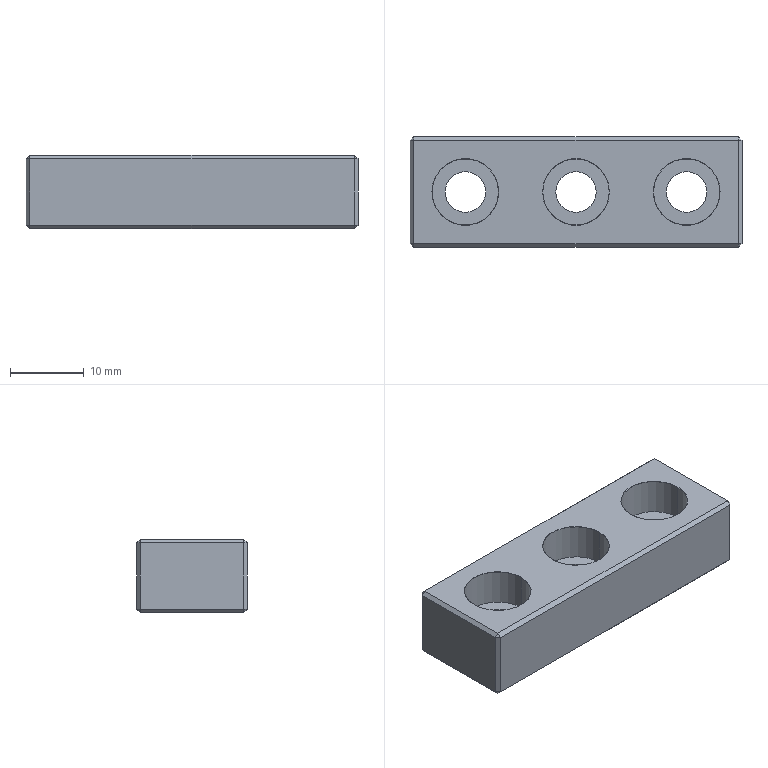Part | SolidWorks | features Chamfer 1, Extrusion 1, HoleWzd 1 | 1 solid | 47 faces | box 45 x 15 x 10 mm | volume 5405 mm3 | plane 29 | cylinder 12 | cone 6 | commonest cylinder face diameters 5.5 x6 9 x6
STEP:
#1=CARTESIAN_POINT('',(10.5,0.,9.976));
#2=VERTEX_POINT('',#1);
#3=CARTESIAN_POINT('',(19.5,0.,9.976));
#4=VERTEX_POINT('',#3);
#5=CARTESIAN_POINT('',(15.,0.,9.976));
#6=DIRECTION('',(0.,0.,1.));
#7=DIRECTION('',(1.,0.,0.));
#8=AXIS2_PLACEMENT_3D('',#5,#6,#7);
#9=CIRCLE('',#8,4.5);
#10=EDGE_CURVE('',#2,#4,#9,.T.);
#11=ORIENTED_EDGE('',*,*,#10,.F.);
#12=CARTESIAN_POINT('',(10.475,0.,10.));
#13=VERTEX_POINT('',#12);
#14=CARTESIAN_POINT('',(10.475,0.,10.));
#15=DIRECTION('',(-0.7193,0.,0.6947));
#16=VECTOR('',#15,1000.);
#17=LINE('',#14,#16);
#18=EDGE_CURVE('',#2,#13,#17,.T.);
#19=ORIENTED_EDGE('',*,*,#18,.T.);
#20=CARTESIAN_POINT('',(19.525,0.,10.));
#21=VERTEX_POINT('',#20);
#22=CARTESIAN_POINT('',(15.,0.,10.));
#23=DIRECTION('',(0.,0.,1.));
#24=DIRECTION('',(1.,0.,0.));
#25=AXIS2_PLACEMENT_3D('',#22,#23,#24);
#26=CIRCLE('',#25,4.525);
#27=EDGE_CURVE('',#13,#21,#26,.T.);
#28=ORIENTED_EDGE('',*,*,#27,.T.);
#29=CARTESIAN_POINT('',(19.525,0.,10.));
#30=DIRECTION('',(0.7193,0.,0.6947));
#31=VECTOR('',#30,1000.);
#32=LINE('',#29,#31);
#33=EDGE_CURVE('',#4,#21,#32,.T.);
#34=ORIENTED_EDGE('',*,*,#33,.F.);
#35=EDGE_LOOP('',(#11,#19,#28,#34));
#36=FACE_OUTER_BOUND('',#35,.T.);
#37=CARTESIAN_POINT('',(15.,0.,10.));
#38=DIRECTION('',(0.,0.,1.));
#39=DIRECTION('',(1.,0.,0.));
#40=AXIS2_PLACEMENT_3D('',#37,#38,#39);
#41=CONICAL_SURFACE('',#40,4.525,0.8029);
#42=ADVANCED_FACE('',(#36),#41,.F.);
#43=CARTESIAN_POINT('',(10.5,0.,5.));
#44=VERTEX_POINT('',#43);
#45=CARTESIAN_POINT('',(19.5,0.,5.));
#46=VERTEX_POINT('',#45);
#47=CARTESIAN_POINT('',(15.,0.,5.));
#48=DIRECTION('',(0.,0.,1.));
#49=DIRECTION('',(1.,0.,0.));
#50=AXIS2_PLACEMENT_3D('',#47,#48,#49);
#51=CIRCLE('',#50,4.5);
#52=EDGE_CURVE('',#44,#46,#51,.T.);
#53=ORIENTED_EDGE('',*,*,#52,.F.);
#54=CARTESIAN_POINT('',(10.5,0.,10.));
#55=DIRECTION('',(0.,0.,1.));
#56=VECTOR('',#55,1000.);
#57=LINE('',#54,#56);
#58=EDGE_CURVE('',#44,#2,#57,.T.);
#59=ORIENTED_EDGE('',*,*,#58,.T.);
#60=ORIENTED_EDGE('',*,*,#10,.T.);
#61=CARTESIAN_POINT('',(19.5,0.,10.));
#62=DIRECTION('',(0.,0.,1.));
#63=VECTOR('',#62,1000.);
#64=LINE('',#61,#63);
#65=EDGE_CURVE('',#46,#4,#64,.T.);
#66=ORIENTED_EDGE('',*,*,#65,.F.);
#67=EDGE_LOOP('',(#53,#59,#60,#66));
#68=FACE_OUTER_BOUND('',#67,.T.);
#69=CARTESIAN_POINT('',(15.,0.,10.));
#70=DIRECTION('',(0.,0.,1.));
#71=DIRECTION('',(1.,0.,0.));
#72=AXIS2_PLACEMENT_3D('',#69,#70,#71);
#73=CYLINDRICAL_SURFACE('',#72,4.5);
#74=ADVANCED_FACE('',(#68),#73,.F.);
#75=CARTESIAN_POINT('',(12.25,0.,0.));
#76=VERTEX_POINT('',#75);
#77=CARTESIAN_POINT('',(17.75,0.,0.));
#78=VERTEX_POINT('',#77);
#79=CARTESIAN_POINT('',(15.,0.,0.));
#80=DIRECTION('',(0.,0.,1.));
#81=DIRECTION('',(1.,0.,0.));
#82=AXIS2_PLACEMENT_3D('',#79,#80,#81);
#83=CIRCLE('',#82,2.75);
#84=EDGE_CURVE('',#76,#78,#83,.T.);
#85=ORIENTED_EDGE('',*,*,#84,.F.);
#86=CARTESIAN_POINT('',(12.25,0.,5.));
#87=VERTEX_POINT('',#86);
#88=CARTESIAN_POINT('',(12.25,0.,10.));
#89=DIRECTION('',(0.,0.,1.));
#90=VECTOR('',#89,1000.);
#91=LINE('',#88,#90);
#92=EDGE_CURVE('',#76,#87,#91,.T.);
#93=ORIENTED_EDGE('',*,*,#92,.T.);
#94=CARTESIAN_POINT('',(17.75,0.,5.));
#95=VERTEX_POINT('',#94);
#96=CARTESIAN_POINT('',(15.,0.,5.));
#97=DIRECTION('',(0.,0.,1.));
#98=DIRECTION('',(1.,0.,0.));
#99=AXIS2_PLACEMENT_3D('',#96,#97,#98);
#100=CIRCLE('',#99,2.75);
#101=EDGE_CURVE('',#87,#95,#100,.T.);
#102=ORIENTED_EDGE('',*,*,#101,.T.);
#103=CARTESIAN_POINT('',(17.75,0.,10.));
#104=DIRECTION('',(0.,0.,1.));
#105=VECTOR('',#104,1000.);
#106=LINE('',#103,#105);
#107=EDGE_CURVE('',#78,#95,#106,.T.);
#108=ORIENTED_EDGE('',*,*,#107,.F.);
#109=EDGE_LOOP('',(#85,#93,#102,#108));
#110=FACE_OUTER_BOUND('',#109,.T.);
#111=CARTESIAN_POINT('',(15.,0.,10.));
#112=DIRECTION('',(0.,0.,1.));
#113=DIRECTION('',(1.,0.,0.));
#114=AXIS2_PLACEMENT_3D('',#111,#112,#113);
#115=CYLINDRICAL_SURFACE('',#114,2.75);
#116=ADVANCED_FACE('',(#110),#115,.F.);
#117=CARTESIAN_POINT('',(-19.5,0.,9.976));
#118=VERTEX_POINT('',#117);
#119=CARTESIAN_POINT('',(-10.5,0.,9.976));
#120=VERTEX_POINT('',#119);
#121=CARTESIAN_POINT('',(-15.,0.,9.976));
#122=DIRECTION('',(0.,0.,1.));
#123=DIRECTION('',(1.,0.,0.));
#124=AXIS2_PLACEMENT_3D('',#121,#122,#123);
#125=CIRCLE('',#124,4.5);
#126=EDGE_CURVE('',#118,#120,#125,.T.);
#127=ORIENTED_EDGE('',*,*,#126,.F.);
#128=CARTESIAN_POINT('',(-19.525,0.,10.));
#129=VERTEX_POINT('',#128);
#130=CARTESIAN_POINT('',(-19.525,0.,10.));
#131=DIRECTION('',(-0.7193,0.,0.6947));
#132=VECTOR('',#131,1000.);
#133=LINE('',#130,#132);
#134=EDGE_CURVE('',#118,#129,#133,.T.);
#135=ORIENTED_EDGE('',*,*,#134,.T.);
#136=CARTESIAN_POINT('',(-10.475,0.,10.));
#137=VERTEX_POINT('',#136);
#138=CARTESIAN_POINT('',(-15.,0.,10.));
#139=DIRECTION('',(0.,0.,1.));
#140=DIRECTION('',(1.,0.,0.));
#141=AXIS2_PLACEMENT_3D('',#138,#139,#140);
#142=CIRCLE('',#141,4.525);
#143=EDGE_CURVE('',#129,#137,#142,.T.);
#144=ORIENTED_EDGE('',*,*,#143,.T.);
#145=CARTESIAN_POINT('',(-10.475,0.,10.));
#146=DIRECTION('',(0.7193,0.,0.6947));
#147=VECTOR('',#146,1000.);
#148=LINE('',#145,#147);
#149=EDGE_CURVE('',#120,#137,#148,.T.);
#150=ORIENTED_EDGE('',*,*,#149,.F.);
#151=EDGE_LOOP('',(#127,#135,#144,#150));
#152=FACE_OUTER_BOUND('',#151,.T.);
#153=CARTESIAN_POINT('',(-15.,0.,10.));
#154=DIRECTION('',(0.,0.,1.));
#155=DIRECTION('',(1.,0.,0.));
#156=AXIS2_PLACEMENT_3D('',#153,#154,#155);
#157=CONICAL_SURFACE('',#156,4.525,0.8029);
#158=ADVANCED_FACE('',(#152),#157,.F.);
#159=CARTESIAN_POINT('',(-19.5,0.,5.));
#160=VERTEX_POINT('',#159);
#161=CARTESIAN_POINT('',(-10.5,0.,5.));
#162=VERTEX_POINT('',#161);
#163=CARTESIAN_POINT('',(-15.,0.,5.));
#164=DIRECTION('',(0.,0.,1.));
#165=DIRECTION('',(1.,0.,0.));
#166=AXIS2_PLACEMENT_3D('',#163,#164,#165);
#167=CIRCLE('',#166,4.5);
#168=EDGE_CURVE('',#160,#162,#167,.T.);
#169=ORIENTED_EDGE('',*,*,#168,.F.);
#170=CARTESIAN_POINT('',(-19.5,0.,10.));
#171=DIRECTION('',(0.,0.,1.));
#172=VECTOR('',#171,1000.);
#173=LINE('',#170,#172);
#174=EDGE_CURVE('',#160,#118,#173,.T.);
#175=ORIENTED_EDGE('',*,*,#174,.T.);
#176=ORIENTED_EDGE('',*,*,#126,.T.);
#177=CARTESIAN_POINT('',(-10.5,0.,10.));
#178=DIRECTION('',(0.,0.,1.));
#179=VECTOR('',#178,1000.);
#180=LINE('',#177,#179);
#181=EDGE_CURVE('',#162,#120,#180,.T.);
#182=ORIENTED_EDGE('',*,*,#181,.F.);
#183=EDGE_LOOP('',(#169,#175,#176,#182));
#184=FACE_OUTER_BOUND('',#183,.T.);
#185=CARTESIAN_POINT('',(-15.,0.,10.));
#186=DIRECTION('',(0.,0.,1.));
#187=DIRECTION('',(1.,0.,0.));
#188=AXIS2_PLACEMENT_3D('',#185,#186,#187);
#189=CYLINDRICAL_SURFACE('',#188,4.5);
#190=ADVANCED_FACE('',(#184),#189,.F.);
#191=CARTESIAN_POINT('',(-17.75,0.,0.));
#192=VERTEX_POINT('',#191);
#193=CARTESIAN_POINT('',(-12.25,0.,0.));
#194=VERTEX_POINT('',#193);
#195=CARTESIAN_POINT('',(-15.,0.,0.));
#196=DIRECTION('',(0.,0.,1.));
#197=DIRECTION('',(1.,0.,0.));
#198=AXIS2_PLACEMENT_3D('',#195,#196,#197);
#199=CIRCLE('',#198,2.75);
#200=EDGE_CURVE('',#192,#194,#199,.T.);
#201=ORIENTED_EDGE('',*,*,#200,.F.);
#202=CARTESIAN_POINT('',(-17.75,0.,5.));
#203=VERTEX_POINT('',#202);
#204=CARTESIAN_POINT('',(-17.75,0.,10.));
#205=DIRECTION('',(0.,0.,1.));
#206=VECTOR('',#205,1000.);
#207=LINE('',#204,#206);
#208=EDGE_CURVE('',#192,#203,#207,.T.);
#209=ORIENTED_EDGE('',*,*,#208,.T.);
#210=CARTESIAN_POINT('',(-12.25,0.,5.));
#211=VERTEX_POINT('',#210);
#212=CARTESIAN_POINT('',(-15.,0.,5.));
#213=DIRECTION('',(0.,0.,1.));
#214=DIRECTION('',(1.,0.,0.));
#215=AXIS2_PLACEMENT_3D('',#212,#213,#214);
#216=CIRCLE('',#215,2.75);
#217=EDGE_CURVE('',#203,#211,#216,.T.);
#218=ORIENTED_EDGE('',*,*,#217,.T.);
#219=CARTESIAN_POINT('',(-12.25,0.,10.));
#220=DIRECTION('',(0.,0.,1.));
#221=VECTOR('',#220,1000.);
#222=LINE('',#219,#221);
#223=EDGE_CURVE('',#194,#211,#222,.T.);
#224=ORIENTED_EDGE('',*,*,#223,.F.);
#225=EDGE_LOOP('',(#201,#209,#218,#224));
#226=FACE_OUTER_BOUND('',#225,.T.);
#227=CARTESIAN_POINT('',(-15.,0.,10.));
#228=DIRECTION('',(0.,0.,1.));
#229=DIRECTION('',(1.,0.,0.));
#230=AXIS2_PLACEMENT_3D('',#227,#228,#229);
#231=CYLINDRICAL_SURFACE('',#230,2.75);
#232=ADVANCED_FACE('',(#226),#231,.F.);
#233=CARTESIAN_POINT('',(-4.5,0.,9.976));
#234=VERTEX_POINT('',#233);
#235=CARTESIAN_POINT('',(4.5,0.,9.976));
#236=VERTEX_POINT('',#235);
#237=CARTESIAN_POINT('',(0.,0.,9.976));
#238=DIRECTION('',(0.,0.,1.));
#239=DIRECTION('',(1.,0.,0.));
#240=AXIS2_PLACEMENT_3D('',#237,#238,#239);
#241=CIRCLE('',#240,4.5);
#242=EDGE_CURVE('',#234,#236,#241,.T.);
#243=ORIENTED_EDGE('',*,*,#242,.F.);
#244=CARTESIAN_POINT('',(-4.525,0.,10.));
#245=VERTEX_POINT('',#244);
#246=CARTESIAN_POINT('',(-4.525,0.,10.));
#247=DIRECTION('',(-0.7193,0.,0.6947));
#248=VECTOR('',#247,1000.);
#249=LINE('',#246,#248);
#250=EDGE_CURVE('',#234,#245,#249,.T.);
#251=ORIENTED_EDGE('',*,*,#250,.T.);
#252=CARTESIAN_POINT('',(4.525,0.,10.));
#253=VERTEX_POINT('',#252);
#254=CARTESIAN_POINT('',(0.,0.,10.));
#255=DIRECTION('',(0.,0.,1.));
#256=DIRECTION('',(1.,0.,0.));
#257=AXIS2_PLACEMENT_3D('',#254,#255,#256);
#258=CIRCLE('',#257,4.525);
#259=EDGE_CURVE('',#245,#253,#258,.T.);
#260=ORIENTED_EDGE('',*,*,#259,.T.);
#261=CARTESIAN_POINT('',(4.525,0.,10.));
#262=DIRECTION('',(0.7193,0.,0.6947));
#263=VECTOR('',#262,1000.);
#264=LINE('',#261,#263);
#265=EDGE_CURVE('',#236,#253,#264,.T.);
#266=ORIENTED_EDGE('',*,*,#265,.F.);
#267=EDGE_LOOP('',(#243,#251,#260,#266));
#268=FACE_OUTER_BOUND('',#267,.T.);
#269=CARTESIAN_POINT('',(0.,0.,10.));
#270=DIRECTION('',(0.,0.,1.));
#271=DIRECTION('',(1.,0.,0.));
#272=AXIS2_PLACEMENT_3D('',#269,#270,#271);
#273=CONICAL_SURFACE('',#272,4.525,0.8029);
#274=ADVANCED_FACE('',(#268),#273,.F.);
#275=CARTESIAN_POINT('',(-4.5,0.,5.));
#276=VERTEX_POINT('',#275);
#277=CARTESIAN_POINT('',(4.5,0.,5.));
#278=VERTEX_POINT('',#277);
#279=CARTESIAN_POINT('',(0.,0.,5.));
#280=DIRECTION('',(0.,0.,1.));
#281=DIRECTION('',(1.,0.,0.));
#282=AXIS2_PLACEMENT_3D('',#279,#280,#281);
#283=CIRCLE('',#282,4.5);
#284=EDGE_CURVE('',#276,#278,#283,.T.);
#285=ORIENTED_EDGE('',*,*,#284,.F.);
#286=CARTESIAN_POINT('',(-4.5,0.,10.));
#287=DIRECTION('',(0.,0.,1.));
#288=VECTOR('',#287,1000.);
#289=LINE('',#286,#288);
#290=EDGE_CURVE('',#276,#234,#289,.T.);
#291=ORIENTED_EDGE('',*,*,#290,.T.);
#292=ORIENTED_EDGE('',*,*,#242,.T.);
#293=CARTESIAN_POINT('',(4.5,0.,10.));
#294=DIRECTION('',(0.,0.,1.));
#295=VECTOR('',#294,1000.);
#296=LINE('',#293,#295);
#297=EDGE_CURVE('',#278,#236,#296,.T.);
#298=ORIENTED_EDGE('',*,*,#297,.F.);
#299=EDGE_LOOP('',(#285,#291,#292,#298));
#300=FACE_OUTER_BOUND('',#299,.T.);
#301=CARTESIAN_POINT('',(0.,0.,10.));
#302=DIRECTION('',(0.,0.,1.));
#303=DIRECTION('',(1.,0.,0.));
#304=AXIS2_PLACEMENT_3D('',#301,#302,#303);
#305=CYLINDRICAL_SURFACE('',#304,4.5);
#306=ADVANCED_FACE('',(#300),#305,.F.);
#307=CARTESIAN_POINT('',(-2.75,0.,0.));
#308=VERTEX_POINT('',#307);
#309=CARTESIAN_POINT('',(2.75,0.,0.));
#310=VERTEX_POINT('',#309);
#311=CARTESIAN_POINT('',(0.,0.,0.));
#312=DIRECTION('',(0.,0.,1.));
#313=DIRECTION('',(1.,0.,0.));
#314=AXIS2_PLACEMENT_3D('',#311,#312,#313);
#315=CIRCLE('',#314,2.75);
#316=EDGE_CURVE('',#308,#310,#315,.T.);
#317=ORIENTED_EDGE('',*,*,#316,.F.);
#318=CARTESIAN_POINT('',(-2.75,0.,5.));
#319=VERTEX_POINT('',#318);
#320=CARTESIAN_POINT('',(-2.75,0.,10.));
#321=DIRECTION('',(0.,0.,1.));
#322=VECTOR('',#321,1000.);
#323=LINE('',#320,#322);
#324=EDGE_CURVE('',#308,#319,#323,.T.);
#325=ORIENTED_EDGE('',*,*,#324,.T.);
#326=CARTESIAN_POINT('',(2.75,0.,5.));
#327=VERTEX_POINT('',#326);
#328=CARTESIAN_POINT('',(0.,0.,5.));
#329=DIRECTION('',(0.,0.,1.));
#330=DIRECTION('',(1.,0.,0.));
#331=AXIS2_PLACEMENT_3D('',#328,#329,#330);
#332=CIRCLE('',#331,2.75);
#333=EDGE_CURVE('',#319,#327,#332,.T.);
#334=ORIENTED_EDGE('',*,*,#333,.T.);
#335=CARTESIAN_POINT('',(2.75,0.,10.));
#336=DIRECTION('',(0.,0.,1.));
#337=VECTOR('',#336,1000.);
#338=LINE('',#335,#337);
#339=EDGE_CURVE('',#310,#327,#338,.T.);
#340=ORIENTED_EDGE('',*,*,#339,.F.);
#341=EDGE_LOOP('',(#317,#325,#334,#340));
#342=FACE_OUTER_BOUND('',#341,.T.);
#343=CARTESIAN_POINT('',(0.,0.,10.));
#344=DIRECTION('',(0.,0.,1.));
#345=DIRECTION('',(1.,0.,0.));
#346=AXIS2_PLACEMENT_3D('',#343,#344,#345);
#347=CYLINDRICAL_SURFACE('',#346,2.75);
#348=ADVANCED_FACE('',(#342),#347,.F.);
#349=CARTESIAN_POINT('',(22.5,7.,0.5));
#350=VERTEX_POINT('',#349);
#351=CARTESIAN_POINT('',(22.5,7.,9.5));
#352=VERTEX_POINT('',#351);
#353=CARTESIAN_POINT('',(22.5,7.,10.));
#354=DIRECTION('',(0.,0.,1.));
#355=VECTOR('',#354,1000.);
#356=LINE('',#353,#355);
#357=EDGE_CURVE('',#350,#352,#356,.T.);
#358=ORIENTED_EDGE('',*,*,#357,.T.);
#359=CARTESIAN_POINT('',(22.5,-7.,9.5));
#360=VERTEX_POINT('',#359);
#361=CARTESIAN_POINT('',(22.5,-7.5,9.5));
#362=DIRECTION('',(0.,-1.,0.));
#363=VECTOR('',#362,1000.);
#364=LINE('',#361,#363);
#365=EDGE_CURVE('',#352,#360,#364,.T.);
#366=ORIENTED_EDGE('',*,*,#365,.T.);
#367=CARTESIAN_POINT('',(22.5,-7.,0.5));
#368=VERTEX_POINT('',#367);
#369=CARTESIAN_POINT('',(22.5,-7.,10.));
#370=DIRECTION('',(0.,0.,-1.));
#371=VECTOR('',#370,1000.);
#372=LINE('',#369,#371);
#373=EDGE_CURVE('',#360,#368,#372,.T.);
#374=ORIENTED_EDGE('',*,*,#373,.T.);
#375=CARTESIAN_POINT('',(22.5,7.5,0.5));
#376=DIRECTION('',(0.,1.,0.));
#377=VECTOR('',#376,1000.);
#378=LINE('',#375,#377);
#379=EDGE_CURVE('',#368,#350,#378,.T.);
#380=ORIENTED_EDGE('',*,*,#379,.T.);
#381=EDGE_LOOP('',(#358,#366,#374,#380));
#382=FACE_OUTER_BOUND('',#381,.T.);
#383=CARTESIAN_POINT('',(22.5,7.5,10.));
#384=DIRECTION('',(-1.,0.,0.));
#385=DIRECTION('',(0.,-1.,0.));
#386=AXIS2_PLACEMENT_3D('',#383,#384,#385);
#387=PLANE('',#386);
#388=ADVANCED_FACE('',(#382),#387,.F.);
#389=CARTESIAN_POINT('',(-22.,7.5,9.5));
#390=VERTEX_POINT('',#389);
#391=CARTESIAN_POINT('',(22.,7.5,9.5));
#392=VERTEX_POINT('',#391);
#393=CARTESIAN_POINT('',(22.5,7.5,9.5));
#394=DIRECTION('',(1.,0.,0.));
#395=VECTOR('',#394,1000.);
#396=LINE('',#393,#395);
#397=EDGE_CURVE('',#390,#392,#396,.T.);
#398=ORIENTED_EDGE('',*,*,#397,.T.);
#399=CARTESIAN_POINT('',(22.,7.5,0.5));
#400=VERTEX_POINT('',#399);
#401=CARTESIAN_POINT('',(22.,7.5,10.));
#402=DIRECTION('',(0.,0.,-1.));
#403=VECTOR('',#402,1000.);
#404=LINE('',#401,#403);
#405=EDGE_CURVE('',#392,#400,#404,.T.);
#406=ORIENTED_EDGE('',*,*,#405,.T.);
#407=CARTESIAN_POINT('',(-22.,7.5,0.5));
#408=VERTEX_POINT('',#407);
#409=CARTESIAN_POINT('',(-22.5,7.5,0.5));
#410=DIRECTION('',(-1.,0.,0.));
#411=VECTOR('',#410,1000.);
#412=LINE('',#409,#411);
#413=EDGE_CURVE('',#400,#408,#412,.T.);
#414=ORIENTED_EDGE('',*,*,#413,.T.);
#415=CARTESIAN_POINT('',(-22.,7.5,10.));
#416=DIRECTION('',(0.,0.,1.));
#417=VECTOR('',#416,1000.);
#418=LINE('',#415,#417);
#419=EDGE_CURVE('',#408,#390,#418,.T.);
#420=ORIENTED_EDGE('',*,*,#419,.T.);
#421=EDGE_LOOP('',(#398,#406,#414,#420));
#422=FACE_OUTER_BOUND('',#421,.T.);
#423=CARTESIAN_POINT('',(-22.5,7.5,10.));
#424=DIRECTION('',(0.,-1.,0.));
#425=DIRECTION('',(0.,0.,-1.));
#426=AXIS2_PLACEMENT_3D('',#423,#424,#425);
#427=PLANE('',#426);
#428=ADVANCED_FACE('',(#422),#427,.F.);
#429=CARTESIAN_POINT('',(-22.5,7.,0.5));
#430=VERTEX_POINT('',#429);
#431=CARTESIAN_POINT('',(-22.5,-7.,0.5));
#432=VERTEX_POINT('',#431);
#433=CARTESIAN_POINT('',(-22.5,7.5,0.5));
#434=DIRECTION('',(0.,-1.,0.));
#435=VECTOR('',#434,1000.);
#436=LINE('',#433,#435);
#437=EDGE_CURVE('',#430,#432,#436,.T.);
#438=ORIENTED_EDGE('',*,*,#437,.T.);
#439=CARTESIAN_POINT('',(-22.5,-7.,9.5));
#440=VERTEX_POINT('',#439);
#441=CARTESIAN_POINT('',(-22.5,-7.,10.));
#442=DIRECTION('',(0.,0.,1.));
#443=VECTOR('',#442,1000.);
#444=LINE('',#441,#443);
#445=EDGE_CURVE('',#432,#440,#444,.T.);
#446=ORIENTED_EDGE('',*,*,#445,.T.);
#447=CARTESIAN_POINT('',(-22.5,7.,9.5));
#448=VERTEX_POINT('',#447);
#449=CARTESIAN_POINT('',(-22.5,7.5,9.5));
#450=DIRECTION('',(0.,1.,0.));
#451=VECTOR('',#450,1000.);
#452=LINE('',#449,#451);
#453=EDGE_CURVE('',#440,#448,#452,.T.);
#454=ORIENTED_EDGE('',*,*,#453,.T.);
#455=CARTESIAN_POINT('',(-22.5,7.,10.));
#456=DIRECTION('',(0.,0.,-1.));
#457=VECTOR('',#456,1000.);
#458=LINE('',#455,#457);
#459=EDGE_CURVE('',#448,#430,#458,.T.);
#460=ORIENTED_EDGE('',*,*,#459,.T.);
#461=EDGE_LOOP('',(#438,#446,#454,#460));
#462=FACE_OUTER_BOUND('',#461,.T.);
#463=CARTESIAN_POINT('',(-22.5,7.5,10.));
#464=DIRECTION('',(1.,0.,0.));
#465=DIRECTION('',(0.,0.,-1.));
#466=AXIS2_PLACEMENT_3D('',#463,#464,#465);
#467=PLANE('',#466);
#468=ADVANCED_FACE('',(#462),#467,.F.);
#469=CARTESIAN_POINT('',(22.,-7.5,9.5));
#470=VERTEX_POINT('',#469);
#471=CARTESIAN_POINT('',(-22.,-7.5,9.5));
#472=VERTEX_POINT('',#471);
#473=CARTESIAN_POINT('',(-22.5,-7.5,9.5));
#474=DIRECTION('',(-1.,0.,0.));
#475=VECTOR('',#474,1000.);
#476=LINE('',#473,#475);
#477=EDGE_CURVE('',#470,#472,#476,.T.);
#478=ORIENTED_EDGE('',*,*,#477,.T.);
#479=CARTESIAN_POINT('',(-22.,-7.5,0.5));
#480=VERTEX_POINT('',#479);
#481=CARTESIAN_POINT('',(-22.,-7.5,10.));
#482=DIRECTION('',(0.,0.,-1.));
#483=VECTOR('',#482,1000.);
#484=LINE('',#481,#483);
#485=EDGE_CURVE('',#472,#480,#484,.T.);
#486=ORIENTED_EDGE('',*,*,#485,.T.);
#487=CARTESIAN_POINT('',(22.,-7.5,0.5));
#488=VERTEX_POINT('',#487);
#489=CARTESIAN_POINT('',(-22.5,-7.5,0.5));
#490=DIRECTION('',(1.,0.,0.));
#491=VECTOR('',#490,1000.);
#492=LINE('',#489,#491);
#493=EDGE_CURVE('',#480,#488,#492,.T.);
#494=ORIENTED_EDGE('',*,*,#493,.T.);
#495=CARTESIAN_POINT('',(22.,-7.5,10.));
#496=DIRECTION('',(0.,0.,1.));
#497=VECTOR('',#496,1000.);
#498=LINE('',#495,#497);
#499=EDGE_CURVE('',#488,#470,#498,.T.);
#500=ORIENTED_EDGE('',*,*,#499,.T.);
#501=EDGE_LOOP('',(#478,#486,#494,#500));
#502=FACE_OUTER_BOUND('',#501,.T.);
#503=CARTESIAN_POINT('',(-22.5,-7.5,10.));
#504=DIRECTION('',(0.,1.,0.));
#505=DIRECTION('',(0.,0.,1.));
#506=AXIS2_PLACEMENT_3D('',#503,#504,#505);
#507=PLANE('',#506);
#508=ADVANCED_FACE('',(#502),#507,.F.);
#509=CARTESIAN_POINT('',(-22.,7.,10.));
#510=VERTEX_POINT('',#509);
#511=CARTESIAN_POINT('',(-22.,-7.,10.));
#512=VERTEX_POINT('',#511);
#513=CARTESIAN_POINT('',(-22.,-7.5,10.));
#514=DIRECTION('',(0.,-1.,0.));
#515=VECTOR('',#514,1000.);
#516=LINE('',#513,#515);
#517=EDGE_CURVE('',#510,#512,#516,.T.);
#518=ORIENTED_EDGE('',*,*,#517,.T.);
#519=CARTESIAN_POINT('',(22.,-7.,10.));
#520=VERTEX_POINT('',#519);
#521=CARTESIAN_POINT('',(22.5,-7.,10.));
#522=DIRECTION('',(1.,0.,0.));
#523=VECTOR('',#522,1000.);
#524=LINE('',#521,#523);
#525=EDGE_CURVE('',#512,#520,#524,.T.);
#526=ORIENTED_EDGE('',*,*,#525,.T.);
#527=CARTESIAN_POINT('',(22.,7.,10.));
#528=VERTEX_POINT('',#527);
#529=CARTESIAN_POINT('',(22.,7.5,10.));
#530=DIRECTION('',(0.,1.,0.));
#531=VECTOR('',#530,1000.);
#532=LINE('',#529,#531);
#533=EDGE_CURVE('',#520,#528,#532,.T.);
#534=ORIENTED_EDGE('',*,*,#533,.T.);
#535=CARTESIAN_POINT('',(-22.5,7.,10.));
#536=DIRECTION('',(-1.,0.,0.));
#537=VECTOR('',#536,1000.);
#538=LINE('',#535,#537);
#539=EDGE_CURVE('',#528,#510,#538,.T.);
#540=ORIENTED_EDGE('',*,*,#539,.T.);
#541=EDGE_LOOP('',(#518,#526,#534,#540));
#542=FACE_OUTER_BOUND('',#541,.T.);
#543=CARTESIAN_POINT('',(15.,0.,10.));
#544=DIRECTION('',(0.,0.,1.));
#545=DIRECTION('',(1.,0.,0.));
#546=AXIS2_PLACEMENT_3D('',#543,#544,#545);
#547=CIRCLE('',#546,4.525);
#548=EDGE_CURVE('',#21,#13,#547,.T.);
#549=ORIENTED_EDGE('',*,*,#548,.F.);
#550=ORIENTED_EDGE('',*,*,#27,.F.);
#551=EDGE_LOOP('',(#549,#550));
#552=FACE_BOUND('',#551,.T.);
#553=CARTESIAN_POINT('',(-15.,0.,10.));
#554=DIRECTION('',(0.,0.,1.));
#555=DIRECTION('',(1.,0.,0.));
#556=AXIS2_PLACEMENT_3D('',#553,#554,#555);
#557=CIRCLE('',#556,4.525);
#558=EDGE_CURVE('',#137,#129,#557,.T.);
#559=ORIENTED_EDGE('',*,*,#558,.F.);
#560=ORIENTED_EDGE('',*,*,#143,.F.);
#561=EDGE_LOOP('',(#559,#560));
#562=FACE_BOUND('',#561,.T.);
#563=CARTESIAN_POINT('',(0.,0.,10.));
#564=DIRECTION('',(0.,0.,1.));
#565=DIRECTION('',(1.,0.,0.));
#566=AXIS2_PLACEMENT_3D('',#563,#564,#565);
#567=CIRCLE('',#566,4.525);
#568=EDGE_CURVE('',#253,#245,#567,.T.);
#569=ORIENTED_EDGE('',*,*,#568,.F.);
#570=ORIENTED_EDGE('',*,*,#259,.F.);
#571=EDGE_LOOP('',(#569,#570));
#572=FACE_BOUND('',#571,.T.);
#573=CARTESIAN_POINT('',(0.,0.,10.));
#574=DIRECTION('',(0.,0.,1.));
#575=DIRECTION('',(1.,0.,0.));
#576=AXIS2_PLACEMENT_3D('',#573,#574,#575);
#577=PLANE('',#576);
#578=ADVANCED_FACE('',(#542,#552,#562,#572),#577,.T.);
#579=CARTESIAN_POINT('',(22.,-7.,0.));
#580=VERTEX_POINT('',#579);
#581=CARTESIAN_POINT('',(-22.,-7.,0.));
#582=VERTEX_POINT('',#581);
#583=CARTESIAN_POINT('',(0.,-7.,0.));
#584=DIRECTION('',(-1.,0.,0.));
#585=VECTOR('',#584,1000.);
#586=LINE('',#583,#585);
#587=EDGE_CURVE('',#580,#582,#586,.T.);
#588=ORIENTED_EDGE('',*,*,#587,.T.);
#589=CARTESIAN_POINT('',(-22.,7.,0.));
#590=VERTEX_POINT('',#589);
#591=CARTESIAN_POINT('',(-22.,0.,0.));
#592=DIRECTION('',(0.,1.,0.));
#593=VECTOR('',#592,1000.);
#594=LINE('',#591,#593);
#595=EDGE_CURVE('',#582,#590,#594,.T.);
#596=ORIENTED_EDGE('',*,*,#595,.T.);
#597=CARTESIAN_POINT('',(22.,7.,0.));
#598=VERTEX_POINT('',#597);
#599=CARTESIAN_POINT('',(0.,7.,0.));
#600=DIRECTION('',(1.,0.,0.));
#601=VECTOR('',#600,1000.);
#602=LINE('',#599,#601);
#603=EDGE_CURVE('',#590,#598,#602,.T.);
#604=ORIENTED_EDGE('',*,*,#603,.T.);
#605=CARTESIAN_POINT('',(22.,0.,0.));
#606=DIRECTION('',(0.,-1.,0.));
#607=VECTOR('',#606,1000.);
#608=LINE('',#605,#607);
#609=EDGE_CURVE('',#598,#580,#608,.T.);
#610=ORIENTED_EDGE('',*,*,#609,.T.);
#611=EDGE_LOOP('',(#588,#596,#604,#610));
#612=FACE_OUTER_BOUND('',#611,.T.);
#613=CARTESIAN_POINT('',(15.,0.,0.));
#614=DIRECTION('',(0.,0.,1.));
#615=DIRECTION('',(1.,0.,0.));
#616=AXIS2_PLACEMENT_3D('',#613,#614,#615);
#617=CIRCLE('',#616,2.75);
#618=EDGE_CURVE('',#78,#76,#617,.T.);
#619=ORIENTED_EDGE('',*,*,#618,.T.);
#620=ORIENTED_EDGE('',*,*,#84,.T.);
#621=EDGE_LOOP('',(#619,#620));
#622=FACE_BOUND('',#621,.T.);
#623=CARTESIAN_POINT('',(-15.,0.,0.));
#624=DIRECTION('',(0.,0.,1.));
#625=DIRECTION('',(1.,0.,0.));
#626=AXIS2_PLACEMENT_3D('',#623,#624,#625);
#627=CIRCLE('',#626,2.75);
#628=EDGE_CURVE('',#194,#192,#627,.T.);
#629=ORIENTED_EDGE('',*,*,#628,.T.);
#630=ORIENTED_EDGE('',*,*,#200,.T.);
#631=EDGE_LOOP('',(#629,#630));
#632=FACE_BOUND('',#631,.T.);
#633=CARTESIAN_POINT('',(0.,0.,0.));
#634=DIRECTION('',(0.,0.,1.));
#635=DIRECTION('',(1.,0.,0.));
#636=AXIS2_PLACEMENT_3D('',#633,#634,#635);
#637=CIRCLE('',#636,2.75);
#638=EDGE_CURVE('',#310,#308,#637,.T.);
#639=ORIENTED_EDGE('',*,*,#638,.T.);
#640=ORIENTED_EDGE('',*,*,#316,.T.);
#641=EDGE_LOOP('',(#639,#640));
#642=FACE_BOUND('',#641,.T.);
#643=CARTESIAN_POINT('',(0.,0.,0.));
#644=DIRECTION('',(0.,0.,1.));
#645=DIRECTION('',(1.,0.,0.));
#646=AXIS2_PLACEMENT_3D('',#643,#644,#645);
#647=PLANE('',#646);
#648=ADVANCED_FACE('',(#612,#622,#632,#642),#647,.F.);
#649=ORIENTED_EDGE('',*,*,#324,.F.);
#650=ORIENTED_EDGE('',*,*,#638,.F.);
#651=ORIENTED_EDGE('',*,*,#339,.T.);
#652=CARTESIAN_POINT('',(0.,0.,5.));
#653=DIRECTION('',(0.,0.,1.));
#654=DIRECTION('',(1.,0.,0.));
#655=AXIS2_PLACEMENT_3D('',#652,#653,#654);
#656=CIRCLE('',#655,2.75);
#657=EDGE_CURVE('',#327,#319,#656,.T.);
#658=ORIENTED_EDGE('',*,*,#657,.T.);
#659=EDGE_LOOP('',(#649,#650,#651,#658));
#660=FACE_OUTER_BOUND('',#659,.T.);
#661=CARTESIAN_POINT('',(0.,0.,10.));
#662=DIRECTION('',(0.,0.,1.));
#663=DIRECTION('',(1.,0.,0.));
#664=AXIS2_PLACEMENT_3D('',#661,#662,#663);
#665=CYLINDRICAL_SURFACE('',#664,2.75);
#666=ADVANCED_FACE('',(#660),#665,.F.);
#667=ORIENTED_EDGE('',*,*,#657,.F.);
#668=ORIENTED_EDGE('',*,*,#333,.F.);
#669=EDGE_LOOP('',(#667,#668));
#670=FACE_BOUND('',#669,.T.);
#671=CARTESIAN_POINT('',(0.,0.,5.));
#672=DIRECTION('',(0.,0.,1.));
#673=DIRECTION('',(1.,0.,0.));
#674=AXIS2_PLACEMENT_3D('',#671,#672,#673);
#675=CIRCLE('',#674,4.5);
#676=EDGE_CURVE('',#278,#276,#675,.T.);
#677=ORIENTED_EDGE('',*,*,#676,.T.);
#678=ORIENTED_EDGE('',*,*,#284,.T.);
#679=EDGE_LOOP('',(#677,#678));
#680=FACE_OUTER_BOUND('',#679,.T.);
#681=CARTESIAN_POINT('',(2.75,0.,5.));
#682=DIRECTION('',(0.,0.,-1.));
#683=DIRECTION('',(-1.,0.,0.));
#684=AXIS2_PLACEMENT_3D('',#681,#682,#683);
#685=PLANE('',#684);
#686=ADVANCED_FACE('',(#670,#680),#685,.F.);
#687=ORIENTED_EDGE('',*,*,#290,.F.);
#688=ORIENTED_EDGE('',*,*,#676,.F.);
#689=ORIENTED_EDGE('',*,*,#297,.T.);
#690=CARTESIAN_POINT('',(0.,0.,9.976));
#691=DIRECTION('',(0.,0.,1.));
#692=DIRECTION('',(1.,0.,0.));
#693=AXIS2_PLACEMENT_3D('',#690,#691,#692);
#694=CIRCLE('',#693,4.5);
#695=EDGE_CURVE('',#236,#234,#694,.T.);
#696=ORIENTED_EDGE('',*,*,#695,.T.);
#697=EDGE_LOOP('',(#687,#688,#689,#696));
#698=FACE_OUTER_BOUND('',#697,.T.);
#699=CARTESIAN_POINT('',(0.,0.,10.));
#700=DIRECTION('',(0.,0.,1.));
#701=DIRECTION('',(1.,0.,0.));
#702=AXIS2_PLACEMENT_3D('',#699,#700,#701);
#703=CYLINDRICAL_SURFACE('',#702,4.5);
#704=ADVANCED_FACE('',(#698),#703,.F.);
#705=ORIENTED_EDGE('',*,*,#250,.F.);
#706=ORIENTED_EDGE('',*,*,#695,.F.);
#707=ORIENTED_EDGE('',*,*,#265,.T.);
#708=ORIENTED_EDGE('',*,*,#568,.T.);
#709=EDGE_LOOP('',(#705,#706,#707,#708));
#710=FACE_OUTER_BOUND('',#709,.T.);
#711=CARTESIAN_POINT('',(0.,0.,10.));
#712=DIRECTION('',(0.,0.,1.));
#713=DIRECTION('',(1.,0.,0.));
#714=AXIS2_PLACEMENT_3D('',#711,#712,#713);
#715=CONICAL_SURFACE('',#714,4.525,0.8029);
#716=ADVANCED_FACE('',(#710),#715,.F.);
#717=ORIENTED_EDGE('',*,*,#208,.F.);
#718=ORIENTED_EDGE('',*,*,#628,.F.);
#719=ORIENTED_EDGE('',*,*,#223,.T.);
#720=CARTESIAN_POINT('',(-15.,0.,5.));
#721=DIRECTION('',(0.,0.,1.));
#722=DIRECTION('',(1.,0.,0.));
#723=AXIS2_PLACEMENT_3D('',#720,#721,#722);
#724=CIRCLE('',#723,2.75);
#725=EDGE_CURVE('',#211,#203,#724,.T.);
#726=ORIENTED_EDGE('',*,*,#725,.T.);
#727=EDGE_LOOP('',(#717,#718,#719,#726));
#728=FACE_OUTER_BOUND('',#727,.T.);
#729=CARTESIAN_POINT('',(-15.,0.,10.));
#730=DIRECTION('',(0.,0.,1.));
#731=DIRECTION('',(1.,0.,0.));
#732=AXIS2_PLACEMENT_3D('',#729,#730,#731);
#733=CYLINDRICAL_SURFACE('',#732,2.75);
#734=ADVANCED_FACE('',(#728),#733,.F.);
#735=ORIENTED_EDGE('',*,*,#725,.F.);
#736=ORIENTED_EDGE('',*,*,#217,.F.);
#737=EDGE_LOOP('',(#735,#736));
#738=FACE_BOUND('',#737,.T.);
#739=CARTESIAN_POINT('',(-15.,0.,5.));
#740=DIRECTION('',(0.,0.,1.));
#741=DIRECTION('',(1.,0.,0.));
#742=AXIS2_PLACEMENT_3D('',#739,#740,#741);
#743=CIRCLE('',#742,4.5);
#744=EDGE_CURVE('',#162,#160,#743,.T.);
#745=ORIENTED_EDGE('',*,*,#744,.T.);
#746=ORIENTED_EDGE('',*,*,#168,.T.);
#747=EDGE_LOOP('',(#745,#746));
#748=FACE_OUTER_BOUND('',#747,.T.);
#749=CARTESIAN_POINT('',(-12.25,0.,5.));
#750=DIRECTION('',(0.,0.,-1.));
#751=DIRECTION('',(-1.,0.,0.));
#752=AXIS2_PLACEMENT_3D('',#749,#750,#751);
#753=PLANE('',#752);
#754=ADVANCED_FACE('',(#738,#748),#753,.F.);
#755=ORIENTED_EDGE('',*,*,#174,.F.);
#756=ORIENTED_EDGE('',*,*,#744,.F.);
#757=ORIENTED_EDGE('',*,*,#181,.T.);
#758=CARTESIAN_POINT('',(-15.,0.,9.976));
#759=DIRECTION('',(0.,0.,1.));
#760=DIRECTION('',(1.,0.,0.));
#761=AXIS2_PLACEMENT_3D('',#758,#759,#760);
#762=CIRCLE('',#761,4.5);
#763=EDGE_CURVE('',#120,#118,#762,.T.);
#764=ORIENTED_EDGE('',*,*,#763,.T.);
#765=EDGE_LOOP('',(#755,#756,#757,#764));
#766=FACE_OUTER_BOUND('',#765,.T.);
#767=CARTESIAN_POINT('',(-15.,0.,10.));
#768=DIRECTION('',(0.,0.,1.));
#769=DIRECTION('',(1.,0.,0.));
#770=AXIS2_PLACEMENT_3D('',#767,#768,#769);
#771=CYLINDRICAL_SURFACE('',#770,4.5);
#772=ADVANCED_FACE('',(#766),#771,.F.);
#773=ORIENTED_EDGE('',*,*,#134,.F.);
#774=ORIENTED_EDGE('',*,*,#763,.F.);
#775=ORIENTED_EDGE('',*,*,#149,.T.);
#776=ORIENTED_EDGE('',*,*,#558,.T.);
#777=EDGE_LOOP('',(#773,#774,#775,#776));
#778=FACE_OUTER_BOUND('',#777,.T.);
#779=CARTESIAN_POINT('',(-15.,0.,10.));
#780=DIRECTION('',(0.,0.,1.));
#781=DIRECTION('',(1.,0.,0.));
#782=AXIS2_PLACEMENT_3D('',#779,#780,#781);
#783=CONICAL_SURFACE('',#782,4.525,0.8029);
#784=ADVANCED_FACE('',(#778),#783,.F.);
#785=ORIENTED_EDGE('',*,*,#92,.F.);
#786=ORIENTED_EDGE('',*,*,#618,.F.);
#787=ORIENTED_EDGE('',*,*,#107,.T.);
#788=CARTESIAN_POINT('',(15.,0.,5.));
#789=DIRECTION('',(0.,0.,1.));
#790=DIRECTION('',(1.,0.,0.));
#791=AXIS2_PLACEMENT_3D('',#788,#789,#790);
#792=CIRCLE('',#791,2.75);
#793=EDGE_CURVE('',#95,#87,#792,.T.);
#794=ORIENTED_EDGE('',*,*,#793,.T.);
#795=EDGE_LOOP('',(#785,#786,#787,#794));
#796=FACE_OUTER_BOUND('',#795,.T.);
#797=CARTESIAN_POINT('',(15.,0.,10.));
#798=DIRECTION('',(0.,0.,1.));
#799=DIRECTION('',(1.,0.,0.));
#800=AXIS2_PLACEMENT_3D('',#797,#798,#799);
#801=CYLINDRICAL_SURFACE('',#800,2.75);
#802=ADVANCED_FACE('',(#796),#801,.F.);
#803=ORIENTED_EDGE('',*,*,#793,.F.);
#804=ORIENTED_EDGE('',*,*,#101,.F.);
#805=EDGE_LOOP('',(#803,#804));
#806=FACE_BOUND('',#805,.T.);
#807=CARTESIAN_POINT('',(15.,0.,5.));
#808=DIRECTION('',(0.,0.,1.));
#809=DIRECTION('',(1.,0.,0.));
#810=AXIS2_PLACEMENT_3D('',#807,#808,#809);
#811=CIRCLE('',#810,4.5);
#812=EDGE_CURVE('',#46,#44,#811,.T.);
#813=ORIENTED_EDGE('',*,*,#812,.T.);
#814=ORIENTED_EDGE('',*,*,#52,.T.);
#815=EDGE_LOOP('',(#813,#814));
#816=FACE_OUTER_BOUND('',#815,.T.);
#817=CARTESIAN_POINT('',(17.75,0.,5.));
#818=DIRECTION('',(0.,0.,-1.));
#819=DIRECTION('',(-1.,0.,0.));
#820=AXIS2_PLACEMENT_3D('',#817,#818,#819);
#821=PLANE('',#820);
#822=ADVANCED_FACE('',(#806,#816),#821,.F.);
#823=ORIENTED_EDGE('',*,*,#58,.F.);
#824=ORIENTED_EDGE('',*,*,#812,.F.);
#825=ORIENTED_EDGE('',*,*,#65,.T.);
#826=CARTESIAN_POINT('',(15.,0.,9.976));
#827=DIRECTION('',(0.,0.,1.));
#828=DIRECTION('',(1.,0.,0.));
#829=AXIS2_PLACEMENT_3D('',#826,#827,#828);
#830=CIRCLE('',#829,4.5);
#831=EDGE_CURVE('',#4,#2,#830,.T.);
#832=ORIENTED_EDGE('',*,*,#831,.T.);
#833=EDGE_LOOP('',(#823,#824,#825,#832));
#834=FACE_OUTER_BOUND('',#833,.T.);
#835=CARTESIAN_POINT('',(15.,0.,10.));
#836=DIRECTION('',(0.,0.,1.));
#837=DIRECTION('',(1.,0.,0.));
#838=AXIS2_PLACEMENT_3D('',#835,#836,#837);
#839=CYLINDRICAL_SURFACE('',#838,4.5);
#840=ADVANCED_FACE('',(#834),#839,.F.);
#841=ORIENTED_EDGE('',*,*,#18,.F.);
#842=ORIENTED_EDGE('',*,*,#831,.F.);
#843=ORIENTED_EDGE('',*,*,#33,.T.);
#844=ORIENTED_EDGE('',*,*,#548,.T.);
#845=EDGE_LOOP('',(#841,#842,#843,#844));
#846=FACE_OUTER_BOUND('',#845,.T.);
#847=CARTESIAN_POINT('',(15.,0.,10.));
#848=DIRECTION('',(0.,0.,1.));
#849=DIRECTION('',(1.,0.,0.));
#850=AXIS2_PLACEMENT_3D('',#847,#848,#849);
#851=CONICAL_SURFACE('',#850,4.525,0.8029);
#852=ADVANCED_FACE('',(#846),#851,.F.);
#853=CARTESIAN_POINT('',(22.5,7.,0.5));
#854=DIRECTION('',(-0.7071,0.,-0.7071));
#855=VECTOR('',#854,1000.);
#856=LINE('',#853,#855);
#857=EDGE_CURVE('',#350,#598,#856,.T.);
#858=ORIENTED_EDGE('',*,*,#857,.F.);
#859=ORIENTED_EDGE('',*,*,#379,.F.);
#860=CARTESIAN_POINT('',(22.5,-7.,0.5));
#861=DIRECTION('',(0.7071,0.,0.7071));
#862=VECTOR('',#861,1000.);
#863=LINE('',#860,#862);
#864=EDGE_CURVE('',#580,#368,#863,.T.);
#865=ORIENTED_EDGE('',*,*,#864,.F.);
#866=ORIENTED_EDGE('',*,*,#609,.F.);
#867=EDGE_LOOP('',(#858,#859,#865,#866));
#868=FACE_OUTER_BOUND('',#867,.T.);
#869=CARTESIAN_POINT('',(22.5,7.5,0.5));
#870=DIRECTION('',(-0.7071,0.,0.7071));
#871=DIRECTION('',(0.,1.,0.));
#872=AXIS2_PLACEMENT_3D('',#869,#870,#871);
#873=PLANE('',#872);
#874=ADVANCED_FACE('',(#868),#873,.F.);
#875=CARTESIAN_POINT('',(22.5,7.,0.5));
#876=DIRECTION('',(-0.7071,0.7071,0.));
#877=VECTOR('',#876,1000.);
#878=LINE('',#875,#877);
#879=EDGE_CURVE('',#350,#400,#878,.T.);
#880=ORIENTED_EDGE('',*,*,#879,.F.);
#881=ORIENTED_EDGE('',*,*,#857,.T.);
#882=CARTESIAN_POINT('',(22.,7.25,0.25));
#883=DIRECTION('',(0.,-0.7071,-0.7071));
#884=VECTOR('',#883,1000.);
#885=LINE('',#882,#884);
#886=EDGE_CURVE('',#400,#598,#885,.T.);
#887=ORIENTED_EDGE('',*,*,#886,.F.);
#888=EDGE_LOOP('',(#880,#881,#887));
#889=FACE_OUTER_BOUND('',#888,.T.);
#890=CARTESIAN_POINT('',(22.5,7.,0.5));
#891=DIRECTION('',(0.5774,0.5774,-0.5774));
#892=DIRECTION('',(-0.7071,0.7071,0.));
#893=AXIS2_PLACEMENT_3D('',#890,#891,#892);
#894=PLANE('',#893);
#895=ADVANCED_FACE('',(#889),#894,.T.);
#896=CARTESIAN_POINT('',(22.,-7.25,0.25));
#897=DIRECTION('',(0.,-0.7071,0.7071));
#898=VECTOR('',#897,1000.);
#899=LINE('',#896,#898);
#900=EDGE_CURVE('',#580,#488,#899,.T.);
#901=ORIENTED_EDGE('',*,*,#900,.F.);
#902=ORIENTED_EDGE('',*,*,#864,.T.);
#903=CARTESIAN_POINT('',(22.5,-7.,0.5));
#904=DIRECTION('',(0.7071,0.7071,0.));
#905=VECTOR('',#904,1000.);
#906=LINE('',#903,#905);
#907=EDGE_CURVE('',#488,#368,#906,.T.);
#908=ORIENTED_EDGE('',*,*,#907,.F.);
#909=EDGE_LOOP('',(#901,#902,#908));
#910=FACE_OUTER_BOUND('',#909,.T.);
#911=CARTESIAN_POINT('',(22.5,-7.,0.5));
#912=DIRECTION('',(0.5774,-0.5774,-0.5774));
#913=DIRECTION('',(0.7071,0.7071,0.));
#914=AXIS2_PLACEMENT_3D('',#911,#912,#913);
#915=PLANE('',#914);
#916=ADVANCED_FACE('',(#910),#915,.T.);
#917=ORIENTED_EDGE('',*,*,#886,.T.);
#918=ORIENTED_EDGE('',*,*,#603,.F.);
#919=CARTESIAN_POINT('',(-22.,7.,0.));
#920=DIRECTION('',(0.,-0.7071,-0.7071));
#921=VECTOR('',#920,1000.);
#922=LINE('',#919,#921);
#923=EDGE_CURVE('',#408,#590,#922,.T.);
#924=ORIENTED_EDGE('',*,*,#923,.F.);
#925=ORIENTED_EDGE('',*,*,#413,.F.);
#926=EDGE_LOOP('',(#917,#918,#924,#925));
#927=FACE_OUTER_BOUND('',#926,.T.);
#928=CARTESIAN_POINT('',(-22.5,7.5,0.5));
#929=DIRECTION('',(0.,-0.7071,0.7071));
#930=DIRECTION('',(-1.,0.,0.));
#931=AXIS2_PLACEMENT_3D('',#928,#929,#930);
#932=PLANE('',#931);
#933=ADVANCED_FACE('',(#927),#932,.F.);
#934=ORIENTED_EDGE('',*,*,#879,.T.);
#935=ORIENTED_EDGE('',*,*,#405,.F.);
#936=CARTESIAN_POINT('',(22.25,7.25,9.5));
#937=DIRECTION('',(-0.7071,0.7071,0.));
#938=VECTOR('',#937,1000.);
#939=LINE('',#936,#938);
#940=EDGE_CURVE('',#352,#392,#939,.T.);
#941=ORIENTED_EDGE('',*,*,#940,.F.);
#942=ORIENTED_EDGE('',*,*,#357,.F.);
#943=EDGE_LOOP('',(#934,#935,#941,#942));
#944=FACE_OUTER_BOUND('',#943,.T.);
#945=CARTESIAN_POINT('',(22.,7.5,10.));
#946=DIRECTION('',(-0.7071,-0.7071,0.));
#947=DIRECTION('',(0.,0.,-1.));
#948=AXIS2_PLACEMENT_3D('',#945,#946,#947);
#949=PLANE('',#948);
#950=ADVANCED_FACE('',(#944),#949,.F.);
#951=CARTESIAN_POINT('',(22.5,-7.,9.5));
#952=DIRECTION('',(-0.7071,0.,0.7071));
#953=VECTOR('',#952,1000.);
#954=LINE('',#951,#953);
#955=EDGE_CURVE('',#360,#520,#954,.T.);
#956=ORIENTED_EDGE('',*,*,#955,.F.);
#957=ORIENTED_EDGE('',*,*,#365,.F.);
#958=CARTESIAN_POINT('',(22.,7.,10.));
#959=DIRECTION('',(0.7071,0.,-0.7071));
#960=VECTOR('',#959,1000.);
#961=LINE('',#958,#960);
#962=EDGE_CURVE('',#528,#352,#961,.T.);
#963=ORIENTED_EDGE('',*,*,#962,.F.);
#964=ORIENTED_EDGE('',*,*,#533,.F.);
#965=EDGE_LOOP('',(#956,#957,#963,#964));
#966=FACE_OUTER_BOUND('',#965,.T.);
#967=CARTESIAN_POINT('',(22.,0.,10.));
#968=DIRECTION('',(0.7071,0.,0.7071));
#969=DIRECTION('',(0.,-1.,0.));
#970=AXIS2_PLACEMENT_3D('',#967,#968,#969);
#971=PLANE('',#970);
#972=ADVANCED_FACE('',(#966),#971,.T.);
#973=ORIENTED_EDGE('',*,*,#907,.T.);
#974=ORIENTED_EDGE('',*,*,#373,.F.);
#975=CARTESIAN_POINT('',(22.5,-7.,9.5));
#976=DIRECTION('',(0.7071,0.7071,0.));
#977=VECTOR('',#976,1000.);
#978=LINE('',#975,#977);
#979=EDGE_CURVE('',#470,#360,#978,.T.);
#980=ORIENTED_EDGE('',*,*,#979,.F.);
#981=ORIENTED_EDGE('',*,*,#499,.F.);
#982=EDGE_LOOP('',(#973,#974,#980,#981));
#983=FACE_OUTER_BOUND('',#982,.T.);
#984=CARTESIAN_POINT('',(22.5,-7.,10.));
#985=DIRECTION('',(-0.7071,0.7071,0.));
#986=DIRECTION('',(0.,0.,-1.));
#987=AXIS2_PLACEMENT_3D('',#984,#985,#986);
#988=PLANE('',#987);
#989=ADVANCED_FACE('',(#983),#988,.F.);
#990=ORIENTED_EDGE('',*,*,#900,.T.);
#991=ORIENTED_EDGE('',*,*,#493,.F.);
#992=CARTESIAN_POINT('',(-22.,-7.25,0.25));
#993=DIRECTION('',(0.,-0.7071,0.7071));
#994=VECTOR('',#993,1000.);
#995=LINE('',#992,#994);
#996=EDGE_CURVE('',#582,#480,#995,.T.);
#997=ORIENTED_EDGE('',*,*,#996,.F.);
#998=ORIENTED_EDGE('',*,*,#587,.F.);
#999=EDGE_LOOP('',(#990,#991,#997,#998));
#1000=FACE_OUTER_BOUND('',#999,.T.);
#1001=CARTESIAN_POINT('',(-22.5,-7.5,0.5));
#1002=DIRECTION('',(0.,0.7071,0.7071));
#1003=DIRECTION('',(1.,0.,0.));
#1004=AXIS2_PLACEMENT_3D('',#1001,#1002,#1003);
#1005=PLANE('',#1004);
#1006=ADVANCED_FACE('',(#1000),#1005,.F.);
#1007=CARTESIAN_POINT('',(-22.,7.,0.));
#1008=DIRECTION('',(-0.7071,0.,0.7071));
#1009=VECTOR('',#1008,1000.);
#1010=LINE('',#1007,#1009);
#1011=EDGE_CURVE('',#590,#430,#1010,.T.);
#1012=ORIENTED_EDGE('',*,*,#1011,.F.);
#1013=ORIENTED_EDGE('',*,*,#595,.F.);
#1014=CARTESIAN_POINT('',(-22.5,-7.,0.5));
#1015=DIRECTION('',(0.7071,0.,-0.7071));
#1016=VECTOR('',#1015,1000.);
#1017=LINE('',#1014,#1016);
#1018=EDGE_CURVE('',#432,#582,#1017,.T.);
#1019=ORIENTED_EDGE('',*,*,#1018,.F.);
#1020=ORIENTED_EDGE('',*,*,#437,.F.);
#1021=EDGE_LOOP('',(#1012,#1013,#1019,#1020));
#1022=FACE_OUTER_BOUND('',#1021,.T.);
#1023=CARTESIAN_POINT('',(-22.5,7.5,0.5));
#1024=DIRECTION('',(0.7071,0.,0.7071));
#1025=DIRECTION('',(0.,-1.,0.));
#1026=AXIS2_PLACEMENT_3D('',#1023,#1024,#1025);
#1027=PLANE('',#1026);
#1028=ADVANCED_FACE('',(#1022),#1027,.F.);
#1029=ORIENTED_EDGE('',*,*,#923,.T.);
#1030=ORIENTED_EDGE('',*,*,#1011,.T.);
#1031=CARTESIAN_POINT('',(-22.25,7.25,0.5));
#1032=DIRECTION('',(-0.7071,-0.7071,0.));
#1033=VECTOR('',#1032,1000.);
#1034=LINE('',#1031,#1033);
#1035=EDGE_CURVE('',#408,#430,#1034,.T.);
#1036=ORIENTED_EDGE('',*,*,#1035,.F.);
#1037=EDGE_LOOP('',(#1029,#1030,#1036));
#1038=FACE_OUTER_BOUND('',#1037,.T.);
#1039=CARTESIAN_POINT('',(-22.,7.,0.));
#1040=DIRECTION('',(-0.5774,0.5774,-0.5774));
#1041=DIRECTION('',(-0.7071,0.,0.7071));
#1042=AXIS2_PLACEMENT_3D('',#1039,#1040,#1041);
#1043=PLANE('',#1042);
#1044=ADVANCED_FACE('',(#1038),#1043,.T.);
#1045=ORIENTED_EDGE('',*,*,#962,.T.);
#1046=ORIENTED_EDGE('',*,*,#940,.T.);
#1047=CARTESIAN_POINT('',(22.,7.,10.));
#1048=DIRECTION('',(0.,0.7071,-0.7071));
#1049=VECTOR('',#1048,1000.);
#1050=LINE('',#1047,#1049);
#1051=EDGE_CURVE('',#528,#392,#1050,.T.);
#1052=ORIENTED_EDGE('',*,*,#1051,.F.);
#1053=EDGE_LOOP('',(#1045,#1046,#1052));
#1054=FACE_OUTER_BOUND('',#1053,.T.);
#1055=CARTESIAN_POINT('',(22.,7.,10.));
#1056=DIRECTION('',(0.5774,0.5774,0.5774));
#1057=DIRECTION('',(-0.7071,0.7071,0.));
#1058=AXIS2_PLACEMENT_3D('',#1055,#1056,#1057);
#1059=PLANE('',#1058);
#1060=ADVANCED_FACE('',(#1054),#1059,.T.);
#1061=ORIENTED_EDGE('',*,*,#979,.T.);
#1062=ORIENTED_EDGE('',*,*,#955,.T.);
#1063=CARTESIAN_POINT('',(22.,-7.25,9.75));
#1064=DIRECTION('',(0.,0.7071,0.7071));
#1065=VECTOR('',#1064,1000.);
#1066=LINE('',#1063,#1065);
#1067=EDGE_CURVE('',#470,#520,#1066,.T.);
#1068=ORIENTED_EDGE('',*,*,#1067,.F.);
#1069=EDGE_LOOP('',(#1061,#1062,#1068));
#1070=FACE_OUTER_BOUND('',#1069,.T.);
#1071=CARTESIAN_POINT('',(22.5,-7.,9.5));
#1072=DIRECTION('',(0.5774,-0.5774,0.5774));
#1073=DIRECTION('',(0.7071,0.7071,0.));
#1074=AXIS2_PLACEMENT_3D('',#1071,#1072,#1073);
#1075=PLANE('',#1074);
#1076=ADVANCED_FACE('',(#1070),#1075,.T.);
#1077=ORIENTED_EDGE('',*,*,#1018,.T.);
#1078=ORIENTED_EDGE('',*,*,#996,.T.);
#1079=CARTESIAN_POINT('',(-22.5,-7.,0.5));
#1080=DIRECTION('',(0.7071,-0.7071,0.));
#1081=VECTOR('',#1080,1000.);
#1082=LINE('',#1079,#1081);
#1083=EDGE_CURVE('',#432,#480,#1082,.T.);
#1084=ORIENTED_EDGE('',*,*,#1083,.F.);
#1085=EDGE_LOOP('',(#1077,#1078,#1084));
#1086=FACE_OUTER_BOUND('',#1085,.T.);
#1087=CARTESIAN_POINT('',(-22.5,-7.,0.5));
#1088=DIRECTION('',(-0.5774,-0.5774,-0.5774));
#1089=DIRECTION('',(-0.7071,0.,0.7071));
#1090=AXIS2_PLACEMENT_3D('',#1087,#1088,#1089);
#1091=PLANE('',#1090);
#1092=ADVANCED_FACE('',(#1086),#1091,.T.);
#1093=ORIENTED_EDGE('',*,*,#1035,.T.);
#1094=ORIENTED_EDGE('',*,*,#459,.F.);
#1095=CARTESIAN_POINT('',(-22.5,7.,9.5));
#1096=DIRECTION('',(-0.7071,-0.7071,0.));
#1097=VECTOR('',#1096,1000.);
#1098=LINE('',#1095,#1097);
#1099=EDGE_CURVE('',#390,#448,#1098,.T.);
#1100=ORIENTED_EDGE('',*,*,#1099,.F.);
#1101=ORIENTED_EDGE('',*,*,#419,.F.);
#1102=EDGE_LOOP('',(#1093,#1094,#1100,#1101));
#1103=FACE_OUTER_BOUND('',#1102,.T.);
#1104=CARTESIAN_POINT('',(-22.5,7.,10.));
#1105=DIRECTION('',(0.7071,-0.7071,0.));
#1106=DIRECTION('',(0.,0.,-1.));
#1107=AXIS2_PLACEMENT_3D('',#1104,#1105,#1106);
#1108=PLANE('',#1107);
#1109=ADVANCED_FACE('',(#1103),#1108,.F.);
#1110=ORIENTED_EDGE('',*,*,#1051,.T.);
#1111=ORIENTED_EDGE('',*,*,#397,.F.);
#1112=CARTESIAN_POINT('',(-22.,7.25,9.75));
#1113=DIRECTION('',(0.,0.7071,-0.7071));
#1114=VECTOR('',#1113,1000.);
#1115=LINE('',#1112,#1114);
#1116=EDGE_CURVE('',#510,#390,#1115,.T.);
#1117=ORIENTED_EDGE('',*,*,#1116,.F.);
#1118=ORIENTED_EDGE('',*,*,#539,.F.);
#1119=EDGE_LOOP('',(#1110,#1111,#1117,#1118));
#1120=FACE_OUTER_BOUND('',#1119,.T.);
#1121=CARTESIAN_POINT('',(0.,7.,10.));
#1122=DIRECTION('',(0.,0.7071,0.7071));
#1123=DIRECTION('',(1.,0.,0.));
#1124=AXIS2_PLACEMENT_3D('',#1121,#1122,#1123);
#1125=PLANE('',#1124);
#1126=ADVANCED_FACE('',(#1120),#1125,.T.);
#1127=ORIENTED_EDGE('',*,*,#1067,.T.);
#1128=ORIENTED_EDGE('',*,*,#525,.F.);
#1129=CARTESIAN_POINT('',(-22.,-7.,10.));
#1130=DIRECTION('',(0.,0.7071,0.7071));
#1131=VECTOR('',#1130,1000.);
#1132=LINE('',#1129,#1131);
#1133=EDGE_CURVE('',#472,#512,#1132,.T.);
#1134=ORIENTED_EDGE('',*,*,#1133,.F.);
#1135=ORIENTED_EDGE('',*,*,#477,.F.);
#1136=EDGE_LOOP('',(#1127,#1128,#1134,#1135));
#1137=FACE_OUTER_BOUND('',#1136,.T.);
#1138=CARTESIAN_POINT('',(0.,-7.,10.));
#1139=DIRECTION('',(0.,-0.7071,0.7071));
#1140=DIRECTION('',(-1.,0.,0.));
#1141=AXIS2_PLACEMENT_3D('',#1138,#1139,#1140);
#1142=PLANE('',#1141);
#1143=ADVANCED_FACE('',(#1137),#1142,.T.);
#1144=ORIENTED_EDGE('',*,*,#1083,.T.);
#1145=ORIENTED_EDGE('',*,*,#485,.F.);
#1146=CARTESIAN_POINT('',(-22.25,-7.25,9.5));
#1147=DIRECTION('',(0.7071,-0.7071,0.));
#1148=VECTOR('',#1147,1000.);
#1149=LINE('',#1146,#1148);
#1150=EDGE_CURVE('',#440,#472,#1149,.T.);
#1151=ORIENTED_EDGE('',*,*,#1150,.F.);
#1152=ORIENTED_EDGE('',*,*,#445,.F.);
#1153=EDGE_LOOP('',(#1144,#1145,#1151,#1152));
#1154=FACE_OUTER_BOUND('',#1153,.T.);
#1155=CARTESIAN_POINT('',(-22.,-7.5,10.));
#1156=DIRECTION('',(0.7071,0.7071,0.));
#1157=DIRECTION('',(0.,0.,-1.));
#1158=AXIS2_PLACEMENT_3D('',#1155,#1156,#1157);
#1159=PLANE('',#1158);
#1160=ADVANCED_FACE('',(#1154),#1159,.F.);
#1161=ORIENTED_EDGE('',*,*,#1116,.T.);
#1162=ORIENTED_EDGE('',*,*,#1099,.T.);
#1163=CARTESIAN_POINT('',(-22.5,7.,9.5));
#1164=DIRECTION('',(-0.7071,0.,-0.7071));
#1165=VECTOR('',#1164,1000.);
#1166=LINE('',#1163,#1165);
#1167=EDGE_CURVE('',#510,#448,#1166,.T.);
#1168=ORIENTED_EDGE('',*,*,#1167,.F.);
#1169=EDGE_LOOP('',(#1161,#1162,#1168));
#1170=FACE_OUTER_BOUND('',#1169,.T.);
#1171=CARTESIAN_POINT('',(-22.5,7.,9.5));
#1172=DIRECTION('',(-0.5774,0.5774,0.5774));
#1173=DIRECTION('',(0.7071,0.,0.7071));
#1174=AXIS2_PLACEMENT_3D('',#1171,#1172,#1173);
#1175=PLANE('',#1174);
#1176=ADVANCED_FACE('',(#1170),#1175,.T.);
#1177=ORIENTED_EDGE('',*,*,#1150,.T.);
#1178=ORIENTED_EDGE('',*,*,#1133,.T.);
#1179=CARTESIAN_POINT('',(-22.,-7.,10.));
#1180=DIRECTION('',(0.7071,0.,0.7071));
#1181=VECTOR('',#1180,1000.);
#1182=LINE('',#1179,#1181);
#1183=EDGE_CURVE('',#440,#512,#1182,.T.);
#1184=ORIENTED_EDGE('',*,*,#1183,.F.);
#1185=EDGE_LOOP('',(#1177,#1178,#1184));
#1186=FACE_OUTER_BOUND('',#1185,.T.);
#1187=CARTESIAN_POINT('',(-22.,-7.,10.));
#1188=DIRECTION('',(-0.5774,-0.5774,0.5774));
#1189=DIRECTION('',(0.7071,0.,0.7071));
#1190=AXIS2_PLACEMENT_3D('',#1187,#1188,#1189);
#1191=PLANE('',#1190);
#1192=ADVANCED_FACE('',(#1186),#1191,.T.);
#1193=ORIENTED_EDGE('',*,*,#1167,.T.);
#1194=ORIENTED_EDGE('',*,*,#453,.F.);
#1195=ORIENTED_EDGE('',*,*,#1183,.T.);
#1196=ORIENTED_EDGE('',*,*,#517,.F.);
#1197=EDGE_LOOP('',(#1193,#1194,#1195,#1196));
#1198=FACE_OUTER_BOUND('',#1197,.T.);
#1199=CARTESIAN_POINT('',(-22.,0.,10.));
#1200=DIRECTION('',(-0.7071,0.,0.7071));
#1201=DIRECTION('',(0.,1.,0.));
#1202=AXIS2_PLACEMENT_3D('',#1199,#1200,#1201);
#1203=PLANE('',#1202);
#1204=ADVANCED_FACE('',(#1198),#1203,.T.);
#1205=CLOSED_SHELL('',(#42,#74,#116,#158,#190,#232,#274,#306,#348,#388,#428,#468,#508,#578,#648,#666,#686,#704,#716,#734,#754,#772,#784,#802,#822,#840,#852,#874,#895,#916,#933,#950,#972,#989,#1006,#1028,#1044,#1060,#1076,#1092,#1109,#1126,#1143,#1160,#1176,#1192,#1204));
#1206=MANIFOLD_SOLID_BREP('',#1205);
#1207=CARTESIAN_POINT('',(0.,0.,0.));
#1208=DIRECTION('',(0.,0.,1.));
#1209=DIRECTION('',(1.,0.,0.));
#1210=AXIS2_PLACEMENT_3D('',#1207,#1208,#1209);
#1211=(LENGTH_UNIT()NAMED_UNIT(*)SI_UNIT(.MILLI.,.METRE.));
#1212=UNCERTAINTY_MEASURE_WITH_UNIT(LENGTH_MEASURE(0.00001),#1211,'','');
#1213=(NAMED_UNIT(*)PLANE_ANGLE_UNIT()SI_UNIT($,.RADIAN.));
#1214=(NAMED_UNIT(*)SI_UNIT($,.STERADIAN.)SOLID_ANGLE_UNIT());
#1215=(GEOMETRIC_REPRESENTATION_CONTEXT(3)GLOBAL_UNCERTAINTY_ASSIGNED_CONTEXT((#1212))GLOBAL_UNIT_ASSIGNED_CONTEXT((#1211,#1213,#1214))REPRESENTATION_CONTEXT('',''));
#1216=ADVANCED_BREP_SHAPE_REPRESENTATION('',(#1206,#1210),#1215);